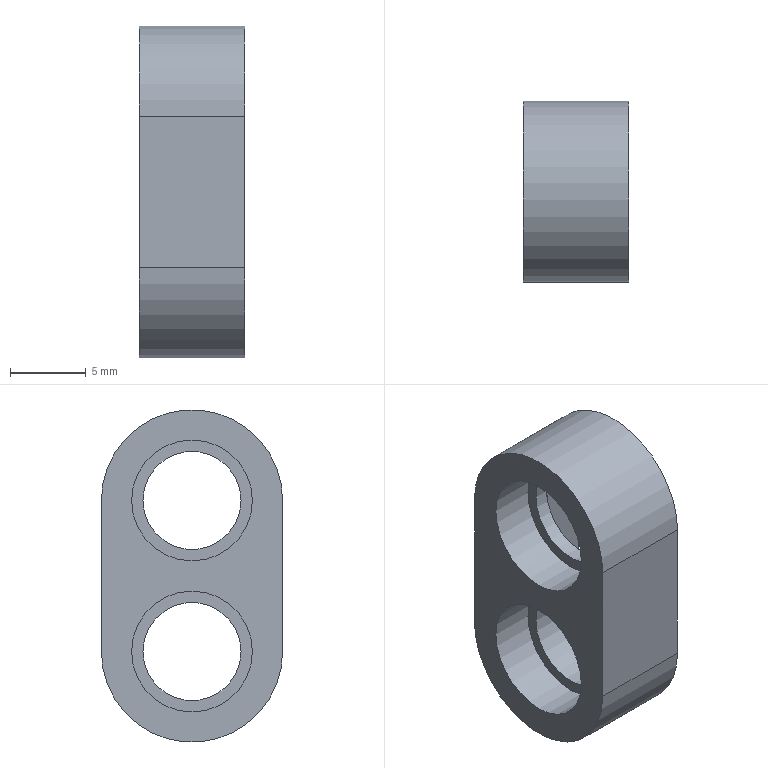Part | STEP file | 1-26.3 | 1 solid | 15 faces | box 7 x 12 x 22 mm | volume 969.173 mm3 | plane 9 | cylinder 6 | commonest cylinder face diameters 6.5 x2 8 x2 12 x2
STEP:
#1=CARTESIAN_POINT('',(0.,0.,0.));
#2=DIRECTION('',(0.,0.,1.));
#3=DIRECTION('',(1.,0.,0.));
#4=AXIS2_PLACEMENT_3D('',#1,#2,#3);
#5=CARTESIAN_POINT('',(0.,6.,5.));
#6=VERTEX_POINT('',#5);
#7=CARTESIAN_POINT('',(-7.,6.,5.));
#8=VERTEX_POINT('',#7);
#9=CARTESIAN_POINT('',(0.,6.,5.));
#10=DIRECTION('',(-1.,0.,0.));
#11=VECTOR('',#10,1.);
#12=LINE('',#9,#11);
#13=CARTESIAN_POINT('',(0.,0.,5.));
#14=DIRECTION('',(-1.,0.,0.));
#15=DIRECTION('',(0.,1.,0.));
#16=AXIS2_PLACEMENT_3D('',#13,#14,#15);
#17=CYLINDRICAL_SURFACE('',#16,6.);
#18=CARTESIAN_POINT('',(6.283,0.));
#19=DIRECTION('',(0.,1.));
#20=VECTOR('',#19,1.);
#21=LINE('',#18,#20);
#22=(GEOMETRIC_REPRESENTATION_CONTEXT(2)PARAMETRIC_REPRESENTATION_CONTEXT()REPRESENTATION_CONTEXT('',''));
#23=DEFINITIONAL_REPRESENTATION('',(#21),#22);
#24=PCURVE('',#17,#23);
#25=CARTESIAN_POINT('',(-3.5,6.,0.));
#26=DIRECTION('',(0.,-1.,0.));
#27=DIRECTION('',(0.,0.,1.));
#28=AXIS2_PLACEMENT_3D('',#25,#26,#27);
#29=PLANE('',#28);
#30=CARTESIAN_POINT('',(5.,-3.5));
#31=DIRECTION('',(0.,1.));
#32=VECTOR('',#31,1.);
#33=LINE('',#30,#32);
#34=(GEOMETRIC_REPRESENTATION_CONTEXT(2)PARAMETRIC_REPRESENTATION_CONTEXT()REPRESENTATION_CONTEXT('',''));
#35=DEFINITIONAL_REPRESENTATION('',(#33),#34);
#36=PCURVE('',#29,#35);
#37=SURFACE_CURVE('',#12,(#24,#36),.PCURVE_S1.);
#38=EDGE_CURVE('',#6,#8,#37,.T.);
#39=ORIENTED_EDGE('',*,*,#38,.T.);
#40=CARTESIAN_POINT('',(-7.,-6.,5.));
#41=VERTEX_POINT('',#40);
#42=CARTESIAN_POINT('',(-7.,0.,5.));
#43=DIRECTION('',(1.,0.,0.));
#44=DIRECTION('',(0.,1.,0.));
#45=AXIS2_PLACEMENT_3D('',#42,#43,#44);
#46=CIRCLE('',#45,6.);
#47=CARTESIAN_POINT('',(6.283,7.));
#48=DIRECTION('',(-1.,0.));
#49=VECTOR('',#48,1.);
#50=LINE('',#47,#49);
#51=(GEOMETRIC_REPRESENTATION_CONTEXT(2)PARAMETRIC_REPRESENTATION_CONTEXT()REPRESENTATION_CONTEXT('',''));
#52=DEFINITIONAL_REPRESENTATION('',(#50),#51);
#53=PCURVE('',#17,#52);
#54=CARTESIAN_POINT('',(-7.,5.,0.));
#55=DIRECTION('',(1.,0.,0.));
#56=DIRECTION('',(0.,0.,-1.));
#57=AXIS2_PLACEMENT_3D('',#54,#55,#56);
#58=PLANE('',#57);
#59=CARTESIAN_POINT('',(-5.,-5.));
#60=DIRECTION('',(0.,1.));
#61=AXIS2_PLACEMENT_2D('',#59,#60);
#62=CIRCLE('',#61,6.);
#63=(GEOMETRIC_REPRESENTATION_CONTEXT(2)PARAMETRIC_REPRESENTATION_CONTEXT()REPRESENTATION_CONTEXT('',''));
#64=DEFINITIONAL_REPRESENTATION('',(#62),#63);
#65=PCURVE('',#58,#64);
#66=SURFACE_CURVE('',#46,(#53,#65),.PCURVE_S1.);
#67=EDGE_CURVE('',#8,#41,#66,.T.);
#68=ORIENTED_EDGE('',*,*,#67,.T.);
#69=CARTESIAN_POINT('',(0.,-6.,5.));
#70=VERTEX_POINT('',#69);
#71=CARTESIAN_POINT('',(0.,-6.,5.));
#72=DIRECTION('',(-1.,0.,0.));
#73=VECTOR('',#72,1.);
#74=LINE('',#71,#73);
#75=CARTESIAN_POINT('',(3.142,0.));
#76=DIRECTION('',(0.,1.));
#77=VECTOR('',#76,1.);
#78=LINE('',#75,#77);
#79=(GEOMETRIC_REPRESENTATION_CONTEXT(2)PARAMETRIC_REPRESENTATION_CONTEXT()REPRESENTATION_CONTEXT('',''));
#80=DEFINITIONAL_REPRESENTATION('',(#78),#79);
#81=PCURVE('',#17,#80);
#82=CARTESIAN_POINT('',(-3.5,-6.,0.));
#83=DIRECTION('',(0.,1.,0.));
#84=DIRECTION('',(0.,0.,-1.));
#85=AXIS2_PLACEMENT_3D('',#82,#83,#84);
#86=PLANE('',#85);
#87=CARTESIAN_POINT('',(-5.,-3.5));
#88=DIRECTION('',(0.,1.));
#89=VECTOR('',#88,1.);
#90=LINE('',#87,#89);
#91=(GEOMETRIC_REPRESENTATION_CONTEXT(2)PARAMETRIC_REPRESENTATION_CONTEXT()REPRESENTATION_CONTEXT('',''));
#92=DEFINITIONAL_REPRESENTATION('',(#90),#91);
#93=PCURVE('',#86,#92);
#94=SURFACE_CURVE('',#74,(#81,#93),.PCURVE_S1.);
#95=EDGE_CURVE('',#70,#41,#94,.T.);
#96=ORIENTED_EDGE('',*,*,#95,.F.);
#97=CARTESIAN_POINT('',(0.,0.,5.));
#98=DIRECTION('',(1.,0.,0.));
#99=DIRECTION('',(0.,1.,0.));
#100=AXIS2_PLACEMENT_3D('',#97,#98,#99);
#101=CIRCLE('',#100,6.);
#102=CARTESIAN_POINT('',(6.283,0.));
#103=DIRECTION('',(-1.,0.));
#104=VECTOR('',#103,1.);
#105=LINE('',#102,#104);
#106=(GEOMETRIC_REPRESENTATION_CONTEXT(2)PARAMETRIC_REPRESENTATION_CONTEXT()REPRESENTATION_CONTEXT('',''));
#107=DEFINITIONAL_REPRESENTATION('',(#105),#106);
#108=PCURVE('',#17,#107);
#109=CARTESIAN_POINT('',(0.,5.,0.));
#110=DIRECTION('',(1.,0.,0.));
#111=DIRECTION('',(0.,0.,-1.));
#112=AXIS2_PLACEMENT_3D('',#109,#110,#111);
#113=PLANE('',#112);
#114=CARTESIAN_POINT('',(-5.,-5.));
#115=DIRECTION('',(0.,1.));
#116=AXIS2_PLACEMENT_2D('',#114,#115);
#117=CIRCLE('',#116,6.);
#118=(GEOMETRIC_REPRESENTATION_CONTEXT(2)PARAMETRIC_REPRESENTATION_CONTEXT()REPRESENTATION_CONTEXT('',''));
#119=DEFINITIONAL_REPRESENTATION('',(#117),#118);
#120=PCURVE('',#113,#119);
#121=SURFACE_CURVE('',#101,(#108,#120),.PCURVE_S1.);
#122=EDGE_CURVE('',#6,#70,#121,.T.);
#123=ORIENTED_EDGE('',*,*,#122,.F.);
#124=EDGE_LOOP('',(#39,#68,#96,#123));
#125=FACE_BOUND('',#124,.T.);
#126=ADVANCED_FACE('',(#125),#17,.T.);
#127=CARTESIAN_POINT('',(0.,-6.,-5.));
#128=VERTEX_POINT('',#127);
#129=CARTESIAN_POINT('',(0.,-6.,5.));
#130=DIRECTION('',(0.,0.,-1.));
#131=VECTOR('',#130,1.);
#132=LINE('',#129,#131);
#133=CARTESIAN_POINT('',(-5.,-3.5));
#134=DIRECTION('',(1.,0.));
#135=VECTOR('',#134,1.);
#136=LINE('',#133,#135);
#137=(GEOMETRIC_REPRESENTATION_CONTEXT(2)PARAMETRIC_REPRESENTATION_CONTEXT()REPRESENTATION_CONTEXT('',''));
#138=DEFINITIONAL_REPRESENTATION('',(#136),#137);
#139=PCURVE('',#86,#138);
#140=CARTESIAN_POINT('',(-5.,-11.));
#141=DIRECTION('',(1.,0.));
#142=VECTOR('',#141,1.);
#143=LINE('',#140,#142);
#144=(GEOMETRIC_REPRESENTATION_CONTEXT(2)PARAMETRIC_REPRESENTATION_CONTEXT()REPRESENTATION_CONTEXT('',''));
#145=DEFINITIONAL_REPRESENTATION('',(#143),#144);
#146=PCURVE('',#113,#145);
#147=SURFACE_CURVE('',#132,(#139,#146),.PCURVE_S1.);
#148=EDGE_CURVE('',#70,#128,#147,.T.);
#149=ORIENTED_EDGE('',*,*,#148,.T.);
#150=CARTESIAN_POINT('',(-7.,-6.,-5.));
#151=VERTEX_POINT('',#150);
#152=CARTESIAN_POINT('',(0.,-6.,-5.));
#153=DIRECTION('',(-1.,0.,0.));
#154=VECTOR('',#153,1.);
#155=LINE('',#152,#154);
#156=CARTESIAN_POINT('',(5.,-3.5));
#157=DIRECTION('',(0.,1.));
#158=VECTOR('',#157,1.);
#159=LINE('',#156,#158);
#160=(GEOMETRIC_REPRESENTATION_CONTEXT(2)PARAMETRIC_REPRESENTATION_CONTEXT()REPRESENTATION_CONTEXT('',''));
#161=DEFINITIONAL_REPRESENTATION('',(#159),#160);
#162=PCURVE('',#86,#161);
#163=CARTESIAN_POINT('',(0.,0.,-5.));
#164=DIRECTION('',(-1.,0.,0.));
#165=DIRECTION('',(0.,-1.,0.));
#166=AXIS2_PLACEMENT_3D('',#163,#164,#165);
#167=CYLINDRICAL_SURFACE('',#166,6.);
#168=CARTESIAN_POINT('',(6.283,0.));
#169=DIRECTION('',(0.,1.));
#170=VECTOR('',#169,1.);
#171=LINE('',#168,#170);
#172=(GEOMETRIC_REPRESENTATION_CONTEXT(2)PARAMETRIC_REPRESENTATION_CONTEXT()REPRESENTATION_CONTEXT('',''));
#173=DEFINITIONAL_REPRESENTATION('',(#171),#172);
#174=PCURVE('',#167,#173);
#175=SURFACE_CURVE('',#155,(#162,#174),.PCURVE_S1.);
#176=EDGE_CURVE('',#128,#151,#175,.T.);
#177=ORIENTED_EDGE('',*,*,#176,.T.);
#178=CARTESIAN_POINT('',(-7.,-6.,5.));
#179=DIRECTION('',(0.,0.,-1.));
#180=VECTOR('',#179,1.);
#181=LINE('',#178,#180);
#182=CARTESIAN_POINT('',(-5.,3.5));
#183=DIRECTION('',(1.,0.));
#184=VECTOR('',#183,1.);
#185=LINE('',#182,#184);
#186=(GEOMETRIC_REPRESENTATION_CONTEXT(2)PARAMETRIC_REPRESENTATION_CONTEXT()REPRESENTATION_CONTEXT('',''));
#187=DEFINITIONAL_REPRESENTATION('',(#185),#186);
#188=PCURVE('',#86,#187);
#189=CARTESIAN_POINT('',(-5.,-11.));
#190=DIRECTION('',(1.,0.));
#191=VECTOR('',#190,1.);
#192=LINE('',#189,#191);
#193=(GEOMETRIC_REPRESENTATION_CONTEXT(2)PARAMETRIC_REPRESENTATION_CONTEXT()REPRESENTATION_CONTEXT('',''));
#194=DEFINITIONAL_REPRESENTATION('',(#192),#193);
#195=PCURVE('',#58,#194);
#196=SURFACE_CURVE('',#181,(#188,#195),.PCURVE_S1.);
#197=EDGE_CURVE('',#41,#151,#196,.T.);
#198=ORIENTED_EDGE('',*,*,#197,.F.);
#199=ORIENTED_EDGE('',*,*,#95,.F.);
#200=EDGE_LOOP('',(#149,#177,#198,#199));
#201=FACE_BOUND('',#200,.F.);
#202=ADVANCED_FACE('',(#201),#86,.F.);
#203=ORIENTED_EDGE('',*,*,#176,.T.);
#204=CARTESIAN_POINT('',(-7.,6.,-5.));
#205=VERTEX_POINT('',#204);
#206=CARTESIAN_POINT('',(-7.,0.,-5.));
#207=DIRECTION('',(1.,0.,0.));
#208=DIRECTION('',(0.,-1.,0.));
#209=AXIS2_PLACEMENT_3D('',#206,#207,#208);
#210=CIRCLE('',#209,6.);
#211=CARTESIAN_POINT('',(6.283,7.));
#212=DIRECTION('',(-1.,0.));
#213=VECTOR('',#212,1.);
#214=LINE('',#211,#213);
#215=(GEOMETRIC_REPRESENTATION_CONTEXT(2)PARAMETRIC_REPRESENTATION_CONTEXT()REPRESENTATION_CONTEXT('',''));
#216=DEFINITIONAL_REPRESENTATION('',(#214),#215);
#217=PCURVE('',#167,#216);
#218=CARTESIAN_POINT('',(5.,-5.));
#219=DIRECTION('',(0.,-1.));
#220=AXIS2_PLACEMENT_2D('',#218,#219);
#221=CIRCLE('',#220,6.);
#222=(GEOMETRIC_REPRESENTATION_CONTEXT(2)PARAMETRIC_REPRESENTATION_CONTEXT()REPRESENTATION_CONTEXT('',''));
#223=DEFINITIONAL_REPRESENTATION('',(#221),#222);
#224=PCURVE('',#58,#223);
#225=SURFACE_CURVE('',#210,(#217,#224),.PCURVE_S1.);
#226=EDGE_CURVE('',#151,#205,#225,.T.);
#227=ORIENTED_EDGE('',*,*,#226,.T.);
#228=CARTESIAN_POINT('',(0.,6.,-5.));
#229=VERTEX_POINT('',#228);
#230=CARTESIAN_POINT('',(0.,6.,-5.));
#231=DIRECTION('',(-1.,0.,0.));
#232=VECTOR('',#231,1.);
#233=LINE('',#230,#232);
#234=CARTESIAN_POINT('',(3.142,0.));
#235=DIRECTION('',(0.,1.));
#236=VECTOR('',#235,1.);
#237=LINE('',#234,#236);
#238=(GEOMETRIC_REPRESENTATION_CONTEXT(2)PARAMETRIC_REPRESENTATION_CONTEXT()REPRESENTATION_CONTEXT('',''));
#239=DEFINITIONAL_REPRESENTATION('',(#237),#238);
#240=PCURVE('',#167,#239);
#241=CARTESIAN_POINT('',(-5.,-3.5));
#242=DIRECTION('',(0.,1.));
#243=VECTOR('',#242,1.);
#244=LINE('',#241,#243);
#245=(GEOMETRIC_REPRESENTATION_CONTEXT(2)PARAMETRIC_REPRESENTATION_CONTEXT()REPRESENTATION_CONTEXT('',''));
#246=DEFINITIONAL_REPRESENTATION('',(#244),#245);
#247=PCURVE('',#29,#246);
#248=SURFACE_CURVE('',#233,(#240,#247),.PCURVE_S1.);
#249=EDGE_CURVE('',#229,#205,#248,.T.);
#250=ORIENTED_EDGE('',*,*,#249,.F.);
#251=CARTESIAN_POINT('',(0.,0.,-5.));
#252=DIRECTION('',(1.,0.,0.));
#253=DIRECTION('',(0.,-1.,0.));
#254=AXIS2_PLACEMENT_3D('',#251,#252,#253);
#255=CIRCLE('',#254,6.);
#256=CARTESIAN_POINT('',(6.283,0.));
#257=DIRECTION('',(-1.,0.));
#258=VECTOR('',#257,1.);
#259=LINE('',#256,#258);
#260=(GEOMETRIC_REPRESENTATION_CONTEXT(2)PARAMETRIC_REPRESENTATION_CONTEXT()REPRESENTATION_CONTEXT('',''));
#261=DEFINITIONAL_REPRESENTATION('',(#259),#260);
#262=PCURVE('',#167,#261);
#263=CARTESIAN_POINT('',(5.,-5.));
#264=DIRECTION('',(0.,-1.));
#265=AXIS2_PLACEMENT_2D('',#263,#264);
#266=CIRCLE('',#265,6.);
#267=(GEOMETRIC_REPRESENTATION_CONTEXT(2)PARAMETRIC_REPRESENTATION_CONTEXT()REPRESENTATION_CONTEXT('',''));
#268=DEFINITIONAL_REPRESENTATION('',(#266),#267);
#269=PCURVE('',#113,#268);
#270=SURFACE_CURVE('',#255,(#262,#269),.PCURVE_S1.);
#271=EDGE_CURVE('',#128,#229,#270,.T.);
#272=ORIENTED_EDGE('',*,*,#271,.F.);
#273=EDGE_LOOP('',(#203,#227,#250,#272));
#274=FACE_BOUND('',#273,.T.);
#275=ADVANCED_FACE('',(#274),#167,.T.);
#276=CARTESIAN_POINT('',(0.,6.,-5.));
#277=DIRECTION('',(0.,0.,1.));
#278=VECTOR('',#277,1.);
#279=LINE('',#276,#278);
#280=CARTESIAN_POINT('',(-5.,-3.5));
#281=DIRECTION('',(1.,0.));
#282=VECTOR('',#281,1.);
#283=LINE('',#280,#282);
#284=(GEOMETRIC_REPRESENTATION_CONTEXT(2)PARAMETRIC_REPRESENTATION_CONTEXT()REPRESENTATION_CONTEXT('',''));
#285=DEFINITIONAL_REPRESENTATION('',(#283),#284);
#286=PCURVE('',#29,#285);
#287=CARTESIAN_POINT('',(5.,1.));
#288=DIRECTION('',(-1.,0.));
#289=VECTOR('',#288,1.);
#290=LINE('',#287,#289);
#291=(GEOMETRIC_REPRESENTATION_CONTEXT(2)PARAMETRIC_REPRESENTATION_CONTEXT()REPRESENTATION_CONTEXT('',''));
#292=DEFINITIONAL_REPRESENTATION('',(#290),#291);
#293=PCURVE('',#113,#292);
#294=SURFACE_CURVE('',#279,(#286,#293),.PCURVE_S1.);
#295=EDGE_CURVE('',#229,#6,#294,.T.);
#296=ORIENTED_EDGE('',*,*,#295,.T.);
#297=ORIENTED_EDGE('',*,*,#38,.T.);
#298=CARTESIAN_POINT('',(-7.,6.,-5.));
#299=DIRECTION('',(0.,0.,1.));
#300=VECTOR('',#299,1.);
#301=LINE('',#298,#300);
#302=CARTESIAN_POINT('',(-5.,3.5));
#303=DIRECTION('',(1.,0.));
#304=VECTOR('',#303,1.);
#305=LINE('',#302,#304);
#306=(GEOMETRIC_REPRESENTATION_CONTEXT(2)PARAMETRIC_REPRESENTATION_CONTEXT()REPRESENTATION_CONTEXT('',''));
#307=DEFINITIONAL_REPRESENTATION('',(#305),#306);
#308=PCURVE('',#29,#307);
#309=CARTESIAN_POINT('',(5.,1.));
#310=DIRECTION('',(-1.,0.));
#311=VECTOR('',#310,1.);
#312=LINE('',#309,#311);
#313=(GEOMETRIC_REPRESENTATION_CONTEXT(2)PARAMETRIC_REPRESENTATION_CONTEXT()REPRESENTATION_CONTEXT('',''));
#314=DEFINITIONAL_REPRESENTATION('',(#312),#313);
#315=PCURVE('',#58,#314);
#316=SURFACE_CURVE('',#301,(#308,#315),.PCURVE_S1.);
#317=EDGE_CURVE('',#205,#8,#316,.T.);
#318=ORIENTED_EDGE('',*,*,#317,.F.);
#319=ORIENTED_EDGE('',*,*,#249,.F.);
#320=EDGE_LOOP('',(#296,#297,#318,#319));
#321=FACE_BOUND('',#320,.F.);
#322=ADVANCED_FACE('',(#321),#29,.F.);
#323=ORIENTED_EDGE('',*,*,#122,.T.);
#324=ORIENTED_EDGE('',*,*,#148,.T.);
#325=ORIENTED_EDGE('',*,*,#271,.T.);
#326=ORIENTED_EDGE('',*,*,#295,.T.);
#327=EDGE_LOOP('',(#323,#324,#325,#326));
#328=FACE_BOUND('',#327,.T.);
#329=CARTESIAN_POINT('',(0.,3.25,-5.));
#330=VERTEX_POINT('',#329);
#331=CARTESIAN_POINT('',(0.,-3.25,-5.));
#332=VERTEX_POINT('',#331);
#333=CARTESIAN_POINT('',(0.,0.,-5.));
#334=DIRECTION('',(-1.,0.,0.));
#335=DIRECTION('',(0.,1.,0.));
#336=AXIS2_PLACEMENT_3D('',#333,#334,#335);
#337=CIRCLE('',#336,3.25);
#338=CARTESIAN_POINT('',(5.,-1.75));
#339=CARTESIAN_POINT('',(10.629,-1.75));
#340=CARTESIAN_POINT('',(7.815,-6.625));
#341=CARTESIAN_POINT('',(5.,-11.5));
#342=CARTESIAN_POINT('',(2.185,-6.625));
#343=CARTESIAN_POINT('',(-0.6292,-1.75));
#344=CARTESIAN_POINT('',(5.,-1.75));
#345=(BOUNDED_CURVE()B_SPLINE_CURVE(2,(#338,#339,#340,#341,#342,#343,#344),.UNSPECIFIED.,.T.,.F.)B_SPLINE_CURVE_WITH_KNOTS((1,2,2,2,2,1),(-2.094,0.,2.094,4.189,6.283,8.378),.UNSPECIFIED.)CURVE()GEOMETRIC_REPRESENTATION_ITEM()RATIONAL_B_SPLINE_CURVE((1.,0.5,1.,0.5,1.,0.5,1.))REPRESENTATION_ITEM(''));
#346=(GEOMETRIC_REPRESENTATION_CONTEXT(2)PARAMETRIC_REPRESENTATION_CONTEXT()REPRESENTATION_CONTEXT('',''));
#347=DEFINITIONAL_REPRESENTATION('',(#345),#346);
#348=PCURVE('',#113,#347);
#349=CARTESIAN_POINT('',(0.,0.,-5.));
#350=DIRECTION('',(-1.,0.,0.));
#351=DIRECTION('',(0.,-1.,0.));
#352=AXIS2_PLACEMENT_3D('',#349,#350,#351);
#353=CYLINDRICAL_SURFACE('',#352,3.25);
#354=CARTESIAN_POINT('',(3.142,0.));
#355=DIRECTION('',(1.,0.));
#356=VECTOR('',#355,1.);
#357=LINE('',#354,#356);
#358=(GEOMETRIC_REPRESENTATION_CONTEXT(2)PARAMETRIC_REPRESENTATION_CONTEXT()REPRESENTATION_CONTEXT('',''));
#359=DEFINITIONAL_REPRESENTATION('',(#357),#358);
#360=PCURVE('',#353,#359);
#361=SURFACE_CURVE('',#337,(#348,#360),.PCURVE_S1.);
#362=EDGE_CURVE('',#330,#332,#361,.T.);
#363=ORIENTED_EDGE('',*,*,#362,.T.);
#364=CARTESIAN_POINT('',(0.,-3.25,5.));
#365=VERTEX_POINT('',#364);
#366=CARTESIAN_POINT('',(0.,-3.25,5.));
#367=DIRECTION('',(0.,0.,-1.));
#368=VECTOR('',#367,1.);
#369=LINE('',#366,#368);
#370=CARTESIAN_POINT('',(-5.,-8.25));
#371=DIRECTION('',(1.,0.));
#372=VECTOR('',#371,1.);
#373=LINE('',#370,#372);
#374=(GEOMETRIC_REPRESENTATION_CONTEXT(2)PARAMETRIC_REPRESENTATION_CONTEXT()REPRESENTATION_CONTEXT('',''));
#375=DEFINITIONAL_REPRESENTATION('',(#373),#374);
#376=PCURVE('',#113,#375);
#377=CARTESIAN_POINT('',(-1.5,-3.25,0.));
#378=DIRECTION('',(0.,1.,0.));
#379=DIRECTION('',(0.,0.,-1.));
#380=AXIS2_PLACEMENT_3D('',#377,#378,#379);
#381=PLANE('',#380);
#382=CARTESIAN_POINT('',(-5.,-1.5));
#383=DIRECTION('',(1.,0.));
#384=VECTOR('',#383,1.);
#385=LINE('',#382,#384);
#386=(GEOMETRIC_REPRESENTATION_CONTEXT(2)PARAMETRIC_REPRESENTATION_CONTEXT()REPRESENTATION_CONTEXT('',''));
#387=DEFINITIONAL_REPRESENTATION('',(#385),#386);
#388=PCURVE('',#381,#387);
#389=SURFACE_CURVE('',#369,(#376,#388),.PCURVE_S1.);
#390=EDGE_CURVE('',#365,#332,#389,.T.);
#391=ORIENTED_EDGE('',*,*,#390,.F.);
#392=CARTESIAN_POINT('',(0.,3.25,5.));
#393=VERTEX_POINT('',#392);
#394=CARTESIAN_POINT('',(0.,0.,5.));
#395=DIRECTION('',(-1.,0.,0.));
#396=DIRECTION('',(0.,-1.,0.));
#397=AXIS2_PLACEMENT_3D('',#394,#395,#396);
#398=CIRCLE('',#397,3.25);
#399=CARTESIAN_POINT('',(-5.,-8.25));
#400=CARTESIAN_POINT('',(-10.629,-8.25));
#401=CARTESIAN_POINT('',(-7.815,-3.375));
#402=CARTESIAN_POINT('',(-5.,1.5));
#403=CARTESIAN_POINT('',(-2.185,-3.375));
#404=CARTESIAN_POINT('',(0.6292,-8.25));
#405=CARTESIAN_POINT('',(-5.,-8.25));
#406=(BOUNDED_CURVE()B_SPLINE_CURVE(2,(#399,#400,#401,#402,#403,#404,#405),.UNSPECIFIED.,.T.,.F.)B_SPLINE_CURVE_WITH_KNOTS((1,2,2,2,2,1),(-2.094,0.,2.094,4.189,6.283,8.378),.UNSPECIFIED.)CURVE()GEOMETRIC_REPRESENTATION_ITEM()RATIONAL_B_SPLINE_CURVE((1.,0.5,1.,0.5,1.,0.5,1.))REPRESENTATION_ITEM(''));
#407=(GEOMETRIC_REPRESENTATION_CONTEXT(2)PARAMETRIC_REPRESENTATION_CONTEXT()REPRESENTATION_CONTEXT('',''));
#408=DEFINITIONAL_REPRESENTATION('',(#406),#407);
#409=PCURVE('',#113,#408);
#410=CARTESIAN_POINT('',(0.,0.,5.));
#411=DIRECTION('',(-1.,0.,0.));
#412=DIRECTION('',(0.,1.,0.));
#413=AXIS2_PLACEMENT_3D('',#410,#411,#412);
#414=CYLINDRICAL_SURFACE('',#413,3.25);
#415=CARTESIAN_POINT('',(3.142,0.));
#416=DIRECTION('',(1.,0.));
#417=VECTOR('',#416,1.);
#418=LINE('',#415,#417);
#419=(GEOMETRIC_REPRESENTATION_CONTEXT(2)PARAMETRIC_REPRESENTATION_CONTEXT()REPRESENTATION_CONTEXT('',''));
#420=DEFINITIONAL_REPRESENTATION('',(#418),#419);
#421=PCURVE('',#414,#420);
#422=SURFACE_CURVE('',#398,(#409,#421),.PCURVE_S1.);
#423=EDGE_CURVE('',#365,#393,#422,.T.);
#424=ORIENTED_EDGE('',*,*,#423,.T.);
#425=CARTESIAN_POINT('',(0.,3.25,-5.));
#426=DIRECTION('',(0.,0.,1.));
#427=VECTOR('',#426,1.);
#428=LINE('',#425,#427);
#429=CARTESIAN_POINT('',(5.,-1.75));
#430=DIRECTION('',(-1.,0.));
#431=VECTOR('',#430,1.);
#432=LINE('',#429,#431);
#433=(GEOMETRIC_REPRESENTATION_CONTEXT(2)PARAMETRIC_REPRESENTATION_CONTEXT()REPRESENTATION_CONTEXT('',''));
#434=DEFINITIONAL_REPRESENTATION('',(#432),#433);
#435=PCURVE('',#113,#434);
#436=CARTESIAN_POINT('',(-1.5,3.25,0.));
#437=DIRECTION('',(0.,-1.,0.));
#438=DIRECTION('',(0.,0.,1.));
#439=AXIS2_PLACEMENT_3D('',#436,#437,#438);
#440=PLANE('',#439);
#441=CARTESIAN_POINT('',(-5.,-1.5));
#442=DIRECTION('',(1.,0.));
#443=VECTOR('',#442,1.);
#444=LINE('',#441,#443);
#445=(GEOMETRIC_REPRESENTATION_CONTEXT(2)PARAMETRIC_REPRESENTATION_CONTEXT()REPRESENTATION_CONTEXT('',''));
#446=DEFINITIONAL_REPRESENTATION('',(#444),#445);
#447=PCURVE('',#440,#446);
#448=SURFACE_CURVE('',#428,(#435,#447),.PCURVE_S1.);
#449=EDGE_CURVE('',#330,#393,#448,.T.);
#450=ORIENTED_EDGE('',*,*,#449,.F.);
#451=EDGE_LOOP('',(#363,#391,#424,#450));
#452=FACE_BOUND('',#451,.T.);
#453=ADVANCED_FACE('',(#328,#452),#113,.T.);
#454=ORIENTED_EDGE('',*,*,#390,.T.);
#455=CARTESIAN_POINT('',(-3.,-3.25,-5.));
#456=VERTEX_POINT('',#455);
#457=CARTESIAN_POINT('',(0.,-3.25,-5.));
#458=DIRECTION('',(-1.,0.,0.));
#459=VECTOR('',#458,1.);
#460=LINE('',#457,#459);
#461=CARTESIAN_POINT('',(5.,-1.5));
#462=DIRECTION('',(0.,1.));
#463=VECTOR('',#462,1.);
#464=LINE('',#461,#463);
#465=(GEOMETRIC_REPRESENTATION_CONTEXT(2)PARAMETRIC_REPRESENTATION_CONTEXT()REPRESENTATION_CONTEXT('',''));
#466=DEFINITIONAL_REPRESENTATION('',(#464),#465);
#467=PCURVE('',#381,#466);
#468=CARTESIAN_POINT('',(6.283,0.));
#469=DIRECTION('',(0.,1.));
#470=VECTOR('',#469,1.);
#471=LINE('',#468,#470);
#472=(GEOMETRIC_REPRESENTATION_CONTEXT(2)PARAMETRIC_REPRESENTATION_CONTEXT()REPRESENTATION_CONTEXT('',''));
#473=DEFINITIONAL_REPRESENTATION('',(#471),#472);
#474=PCURVE('',#353,#473);
#475=SURFACE_CURVE('',#460,(#467,#474),.PCURVE_S1.);
#476=EDGE_CURVE('',#332,#456,#475,.T.);
#477=ORIENTED_EDGE('',*,*,#476,.T.);
#478=CARTESIAN_POINT('',(-3.,-3.25,5.));
#479=VERTEX_POINT('',#478);
#480=CARTESIAN_POINT('',(-3.,-3.25,5.));
#481=DIRECTION('',(0.,0.,-1.));
#482=VECTOR('',#481,1.);
#483=LINE('',#480,#482);
#484=CARTESIAN_POINT('',(-5.,1.5));
#485=DIRECTION('',(1.,0.));
#486=VECTOR('',#485,1.);
#487=LINE('',#484,#486);
#488=(GEOMETRIC_REPRESENTATION_CONTEXT(2)PARAMETRIC_REPRESENTATION_CONTEXT()REPRESENTATION_CONTEXT('',''));
#489=DEFINITIONAL_REPRESENTATION('',(#487),#488);
#490=PCURVE('',#381,#489);
#491=CARTESIAN_POINT('',(-3.,5.,0.));
#492=DIRECTION('',(1.,0.,0.));
#493=DIRECTION('',(0.,0.,-1.));
#494=AXIS2_PLACEMENT_3D('',#491,#492,#493);
#495=PLANE('',#494);
#496=CARTESIAN_POINT('',(-5.,-8.25));
#497=DIRECTION('',(1.,0.));
#498=VECTOR('',#497,1.);
#499=LINE('',#496,#498);
#500=(GEOMETRIC_REPRESENTATION_CONTEXT(2)PARAMETRIC_REPRESENTATION_CONTEXT()REPRESENTATION_CONTEXT('',''));
#501=DEFINITIONAL_REPRESENTATION('',(#499),#500);
#502=PCURVE('',#495,#501);
#503=SURFACE_CURVE('',#483,(#490,#502),.PCURVE_S1.);
#504=EDGE_CURVE('',#479,#456,#503,.T.);
#505=ORIENTED_EDGE('',*,*,#504,.F.);
#506=CARTESIAN_POINT('',(0.,-3.25,5.));
#507=DIRECTION('',(-1.,0.,0.));
#508=VECTOR('',#507,1.);
#509=LINE('',#506,#508);
#510=CARTESIAN_POINT('',(-5.,-1.5));
#511=DIRECTION('',(0.,1.));
#512=VECTOR('',#511,1.);
#513=LINE('',#510,#512);
#514=(GEOMETRIC_REPRESENTATION_CONTEXT(2)PARAMETRIC_REPRESENTATION_CONTEXT()REPRESENTATION_CONTEXT('',''));
#515=DEFINITIONAL_REPRESENTATION('',(#513),#514);
#516=PCURVE('',#381,#515);
#517=CARTESIAN_POINT('',(3.142,0.));
#518=DIRECTION('',(0.,1.));
#519=VECTOR('',#518,1.);
#520=LINE('',#517,#519);
#521=(GEOMETRIC_REPRESENTATION_CONTEXT(2)PARAMETRIC_REPRESENTATION_CONTEXT()REPRESENTATION_CONTEXT('',''));
#522=DEFINITIONAL_REPRESENTATION('',(#520),#521);
#523=PCURVE('',#414,#522);
#524=SURFACE_CURVE('',#509,(#516,#523),.PCURVE_S1.);
#525=EDGE_CURVE('',#365,#479,#524,.T.);
#526=ORIENTED_EDGE('',*,*,#525,.F.);
#527=EDGE_LOOP('',(#454,#477,#505,#526));
#528=FACE_BOUND('',#527,.T.);
#529=ADVANCED_FACE('',(#528),#381,.T.);
#530=ORIENTED_EDGE('',*,*,#449,.T.);
#531=CARTESIAN_POINT('',(-3.,3.25,5.));
#532=VERTEX_POINT('',#531);
#533=CARTESIAN_POINT('',(0.,3.25,5.));
#534=DIRECTION('',(-1.,0.,0.));
#535=VECTOR('',#534,1.);
#536=LINE('',#533,#535);
#537=CARTESIAN_POINT('',(5.,-1.5));
#538=DIRECTION('',(0.,1.));
#539=VECTOR('',#538,1.);
#540=LINE('',#537,#539);
#541=(GEOMETRIC_REPRESENTATION_CONTEXT(2)PARAMETRIC_REPRESENTATION_CONTEXT()REPRESENTATION_CONTEXT('',''));
#542=DEFINITIONAL_REPRESENTATION('',(#540),#541);
#543=PCURVE('',#440,#542);
#544=CARTESIAN_POINT('',(6.283,0.));
#545=DIRECTION('',(0.,1.));
#546=VECTOR('',#545,1.);
#547=LINE('',#544,#546);
#548=(GEOMETRIC_REPRESENTATION_CONTEXT(2)PARAMETRIC_REPRESENTATION_CONTEXT()REPRESENTATION_CONTEXT('',''));
#549=DEFINITIONAL_REPRESENTATION('',(#547),#548);
#550=PCURVE('',#414,#549);
#551=SURFACE_CURVE('',#536,(#543,#550),.PCURVE_S1.);
#552=EDGE_CURVE('',#393,#532,#551,.T.);
#553=ORIENTED_EDGE('',*,*,#552,.T.);
#554=CARTESIAN_POINT('',(-3.,3.25,-5.));
#555=VERTEX_POINT('',#554);
#556=CARTESIAN_POINT('',(-3.,3.25,-5.));
#557=DIRECTION('',(0.,0.,1.));
#558=VECTOR('',#557,1.);
#559=LINE('',#556,#558);
#560=CARTESIAN_POINT('',(-5.,1.5));
#561=DIRECTION('',(1.,0.));
#562=VECTOR('',#561,1.);
#563=LINE('',#560,#562);
#564=(GEOMETRIC_REPRESENTATION_CONTEXT(2)PARAMETRIC_REPRESENTATION_CONTEXT()REPRESENTATION_CONTEXT('',''));
#565=DEFINITIONAL_REPRESENTATION('',(#563),#564);
#566=PCURVE('',#440,#565);
#567=CARTESIAN_POINT('',(5.,-1.75));
#568=DIRECTION('',(-1.,0.));
#569=VECTOR('',#568,1.);
#570=LINE('',#567,#569);
#571=(GEOMETRIC_REPRESENTATION_CONTEXT(2)PARAMETRIC_REPRESENTATION_CONTEXT()REPRESENTATION_CONTEXT('',''));
#572=DEFINITIONAL_REPRESENTATION('',(#570),#571);
#573=PCURVE('',#495,#572);
#574=SURFACE_CURVE('',#559,(#566,#573),.PCURVE_S1.);
#575=EDGE_CURVE('',#555,#532,#574,.T.);
#576=ORIENTED_EDGE('',*,*,#575,.F.);
#577=CARTESIAN_POINT('',(0.,3.25,-5.));
#578=DIRECTION('',(-1.,0.,0.));
#579=VECTOR('',#578,1.);
#580=LINE('',#577,#579);
#581=CARTESIAN_POINT('',(-5.,-1.5));
#582=DIRECTION('',(0.,1.));
#583=VECTOR('',#582,1.);
#584=LINE('',#581,#583);
#585=(GEOMETRIC_REPRESENTATION_CONTEXT(2)PARAMETRIC_REPRESENTATION_CONTEXT()REPRESENTATION_CONTEXT('',''));
#586=DEFINITIONAL_REPRESENTATION('',(#584),#585);
#587=PCURVE('',#440,#586);
#588=CARTESIAN_POINT('',(3.142,0.));
#589=DIRECTION('',(0.,1.));
#590=VECTOR('',#589,1.);
#591=LINE('',#588,#590);
#592=(GEOMETRIC_REPRESENTATION_CONTEXT(2)PARAMETRIC_REPRESENTATION_CONTEXT()REPRESENTATION_CONTEXT('',''));
#593=DEFINITIONAL_REPRESENTATION('',(#591),#592);
#594=PCURVE('',#353,#593);
#595=SURFACE_CURVE('',#580,(#587,#594),.PCURVE_S1.);
#596=EDGE_CURVE('',#330,#555,#595,.T.);
#597=ORIENTED_EDGE('',*,*,#596,.F.);
#598=EDGE_LOOP('',(#530,#553,#576,#597));
#599=FACE_BOUND('',#598,.T.);
#600=ADVANCED_FACE('',(#599),#440,.T.);
#601=ORIENTED_EDGE('',*,*,#504,.T.);
#602=CARTESIAN_POINT('',(-3.,0.,-5.));
#603=DIRECTION('',(-1.,0.,0.));
#604=DIRECTION('',(0.,-1.,0.));
#605=AXIS2_PLACEMENT_3D('',#602,#603,#604);
#606=CIRCLE('',#605,3.25);
#607=CARTESIAN_POINT('',(5.,-8.25));
#608=CARTESIAN_POINT('',(-0.6292,-8.25));
#609=CARTESIAN_POINT('',(2.185,-3.375));
#610=CARTESIAN_POINT('',(5.,1.5));
#611=CARTESIAN_POINT('',(7.815,-3.375));
#612=CARTESIAN_POINT('',(10.629,-8.25));
#613=CARTESIAN_POINT('',(5.,-8.25));
#614=(BOUNDED_CURVE()B_SPLINE_CURVE(2,(#607,#608,#609,#610,#611,#612,#613),.UNSPECIFIED.,.T.,.F.)B_SPLINE_CURVE_WITH_KNOTS((1,2,2,2,2,1),(-2.094,0.,2.094,4.189,6.283,8.378),.UNSPECIFIED.)CURVE()GEOMETRIC_REPRESENTATION_ITEM()RATIONAL_B_SPLINE_CURVE((1.,0.5,1.,0.5,1.,0.5,1.))REPRESENTATION_ITEM(''));
#615=(GEOMETRIC_REPRESENTATION_CONTEXT(2)PARAMETRIC_REPRESENTATION_CONTEXT()REPRESENTATION_CONTEXT('',''));
#616=DEFINITIONAL_REPRESENTATION('',(#614),#615);
#617=PCURVE('',#495,#616);
#618=CARTESIAN_POINT('',(0.,3.));
#619=DIRECTION('',(1.,0.));
#620=VECTOR('',#619,1.);
#621=LINE('',#618,#620);
#622=(GEOMETRIC_REPRESENTATION_CONTEXT(2)PARAMETRIC_REPRESENTATION_CONTEXT()REPRESENTATION_CONTEXT('',''));
#623=DEFINITIONAL_REPRESENTATION('',(#621),#622);
#624=PCURVE('',#353,#623);
#625=SURFACE_CURVE('',#606,(#617,#624),.PCURVE_S1.);
#626=EDGE_CURVE('',#456,#555,#625,.T.);
#627=ORIENTED_EDGE('',*,*,#626,.T.);
#628=ORIENTED_EDGE('',*,*,#575,.T.);
#629=CARTESIAN_POINT('',(-3.,0.,5.));
#630=DIRECTION('',(-1.,0.,0.));
#631=DIRECTION('',(0.,1.,0.));
#632=AXIS2_PLACEMENT_3D('',#629,#630,#631);
#633=CIRCLE('',#632,3.25);
#634=CARTESIAN_POINT('',(-5.,-1.75));
#635=CARTESIAN_POINT('',(0.6292,-1.75));
#636=CARTESIAN_POINT('',(-2.185,-6.625));
#637=CARTESIAN_POINT('',(-5.,-11.5));
#638=CARTESIAN_POINT('',(-7.815,-6.625));
#639=CARTESIAN_POINT('',(-10.629,-1.75));
#640=CARTESIAN_POINT('',(-5.,-1.75));
#641=(BOUNDED_CURVE()B_SPLINE_CURVE(2,(#634,#635,#636,#637,#638,#639,#640),.UNSPECIFIED.,.T.,.F.)B_SPLINE_CURVE_WITH_KNOTS((1,2,2,2,2,1),(-2.094,0.,2.094,4.189,6.283,8.378),.UNSPECIFIED.)CURVE()GEOMETRIC_REPRESENTATION_ITEM()RATIONAL_B_SPLINE_CURVE((1.,0.5,1.,0.5,1.,0.5,1.))REPRESENTATION_ITEM(''));
#642=(GEOMETRIC_REPRESENTATION_CONTEXT(2)PARAMETRIC_REPRESENTATION_CONTEXT()REPRESENTATION_CONTEXT('',''));
#643=DEFINITIONAL_REPRESENTATION('',(#641),#642);
#644=PCURVE('',#495,#643);
#645=CARTESIAN_POINT('',(0.,3.));
#646=DIRECTION('',(1.,0.));
#647=VECTOR('',#646,1.);
#648=LINE('',#645,#647);
#649=(GEOMETRIC_REPRESENTATION_CONTEXT(2)PARAMETRIC_REPRESENTATION_CONTEXT()REPRESENTATION_CONTEXT('',''));
#650=DEFINITIONAL_REPRESENTATION('',(#648),#649);
#651=PCURVE('',#414,#650);
#652=SURFACE_CURVE('',#633,(#644,#651),.PCURVE_S1.);
#653=EDGE_CURVE('',#532,#479,#652,.T.);
#654=ORIENTED_EDGE('',*,*,#653,.T.);
#655=EDGE_LOOP('',(#601,#627,#628,#654));
#656=FACE_BOUND('',#655,.T.);
#657=ADVANCED_FACE('',(#656),#495,.T.);
#658=ORIENTED_EDGE('',*,*,#67,.T.);
#659=ORIENTED_EDGE('',*,*,#197,.T.);
#660=ORIENTED_EDGE('',*,*,#226,.T.);
#661=ORIENTED_EDGE('',*,*,#317,.T.);
#662=EDGE_LOOP('',(#658,#659,#660,#661));
#663=FACE_BOUND('',#662,.F.);
#664=CARTESIAN_POINT('',(-7.,-4.,5.));
#665=VERTEX_POINT('',#664);
#666=CARTESIAN_POINT('',(-7.,0.,5.));
#667=DIRECTION('',(-1.,0.,0.));
#668=DIRECTION('',(0.,-1.,0.));
#669=AXIS2_PLACEMENT_3D('',#666,#667,#668);
#670=CIRCLE('',#669,4.);
#671=CARTESIAN_POINT('',(-5.,-9.));
#672=CARTESIAN_POINT('',(-11.928,-9.));
#673=CARTESIAN_POINT('',(-8.464,-3.));
#674=CARTESIAN_POINT('',(-5.,3.));
#675=CARTESIAN_POINT('',(-1.536,-3.));
#676=CARTESIAN_POINT('',(1.928,-9.));
#677=CARTESIAN_POINT('',(-5.,-9.));
#678=(BOUNDED_CURVE()B_SPLINE_CURVE(2,(#671,#672,#673,#674,#675,#676,#677),.UNSPECIFIED.,.T.,.F.)B_SPLINE_CURVE_WITH_KNOTS((1,2,2,2,2,1),(-2.094,0.,2.094,4.189,6.283,8.378),.UNSPECIFIED.)CURVE()GEOMETRIC_REPRESENTATION_ITEM()RATIONAL_B_SPLINE_CURVE((1.,0.5,1.,0.5,1.,0.5,1.))REPRESENTATION_ITEM(''));
#679=(GEOMETRIC_REPRESENTATION_CONTEXT(2)PARAMETRIC_REPRESENTATION_CONTEXT()REPRESENTATION_CONTEXT('',''));
#680=DEFINITIONAL_REPRESENTATION('',(#678),#679);
#681=PCURVE('',#58,#680);
#682=CARTESIAN_POINT('',(-7.,0.,5.));
#683=DIRECTION('',(1.,0.,0.));
#684=DIRECTION('',(0.,-1.,0.));
#685=AXIS2_PLACEMENT_3D('',#682,#683,#684);
#686=CYLINDRICAL_SURFACE('',#685,4.);
#687=CARTESIAN_POINT('',(6.283,0.));
#688=DIRECTION('',(-1.,0.));
#689=VECTOR('',#688,1.);
#690=LINE('',#687,#689);
#691=(GEOMETRIC_REPRESENTATION_CONTEXT(2)PARAMETRIC_REPRESENTATION_CONTEXT()REPRESENTATION_CONTEXT('',''));
#692=DEFINITIONAL_REPRESENTATION('',(#690),#691);
#693=PCURVE('',#686,#692);
#694=SURFACE_CURVE('',#670,(#681,#693),.PCURVE_S1.);
#695=EDGE_CURVE('',#665,#665,#694,.T.);
#696=ORIENTED_EDGE('',*,*,#695,.T.);
#697=EDGE_LOOP('',(#696));
#698=FACE_BOUND('',#697,.F.);
#699=CARTESIAN_POINT('',(-7.,-4.,-5.));
#700=VERTEX_POINT('',#699);
#701=CARTESIAN_POINT('',(-7.,0.,-5.));
#702=DIRECTION('',(-1.,0.,0.));
#703=DIRECTION('',(0.,-1.,0.));
#704=AXIS2_PLACEMENT_3D('',#701,#702,#703);
#705=CIRCLE('',#704,4.);
#706=CARTESIAN_POINT('',(5.,-9.));
#707=CARTESIAN_POINT('',(-1.928,-9.));
#708=CARTESIAN_POINT('',(1.536,-3.));
#709=CARTESIAN_POINT('',(5.,3.));
#710=CARTESIAN_POINT('',(8.464,-3.));
#711=CARTESIAN_POINT('',(11.928,-9.));
#712=CARTESIAN_POINT('',(5.,-9.));
#713=(BOUNDED_CURVE()B_SPLINE_CURVE(2,(#706,#707,#708,#709,#710,#711,#712),.UNSPECIFIED.,.T.,.F.)B_SPLINE_CURVE_WITH_KNOTS((1,2,2,2,2,1),(-2.094,0.,2.094,4.189,6.283,8.378),.UNSPECIFIED.)CURVE()GEOMETRIC_REPRESENTATION_ITEM()RATIONAL_B_SPLINE_CURVE((1.,0.5,1.,0.5,1.,0.5,1.))REPRESENTATION_ITEM(''));
#714=(GEOMETRIC_REPRESENTATION_CONTEXT(2)PARAMETRIC_REPRESENTATION_CONTEXT()REPRESENTATION_CONTEXT('',''));
#715=DEFINITIONAL_REPRESENTATION('',(#713),#714);
#716=PCURVE('',#58,#715);
#717=CARTESIAN_POINT('',(-7.,0.,-5.));
#718=DIRECTION('',(1.,0.,0.));
#719=DIRECTION('',(0.,-1.,0.));
#720=AXIS2_PLACEMENT_3D('',#717,#718,#719);
#721=CYLINDRICAL_SURFACE('',#720,4.);
#722=CARTESIAN_POINT('',(6.283,0.));
#723=DIRECTION('',(-1.,0.));
#724=VECTOR('',#723,1.);
#725=LINE('',#722,#724);
#726=(GEOMETRIC_REPRESENTATION_CONTEXT(2)PARAMETRIC_REPRESENTATION_CONTEXT()REPRESENTATION_CONTEXT('',''));
#727=DEFINITIONAL_REPRESENTATION('',(#725),#726);
#728=PCURVE('',#721,#727);
#729=SURFACE_CURVE('',#705,(#716,#728),.PCURVE_S1.);
#730=EDGE_CURVE('',#700,#700,#729,.T.);
#731=ORIENTED_EDGE('',*,*,#730,.T.);
#732=EDGE_LOOP('',(#731));
#733=FACE_BOUND('',#732,.F.);
#734=ADVANCED_FACE('',(#663,#698,#733),#58,.F.);
#735=CARTESIAN_POINT('',(-4.,-3.25,-5.));
#736=VERTEX_POINT('',#735);
#737=CARTESIAN_POINT('',(-3.,-3.25,-5.));
#738=DIRECTION('',(-1.,0.,0.));
#739=VECTOR('',#738,1.);
#740=LINE('',#737,#739);
#741=CARTESIAN_POINT('',(6.283,3.));
#742=DIRECTION('',(0.,1.));
#743=VECTOR('',#742,1.);
#744=LINE('',#741,#743);
#745=(GEOMETRIC_REPRESENTATION_CONTEXT(2)PARAMETRIC_REPRESENTATION_CONTEXT()REPRESENTATION_CONTEXT('',''));
#746=DEFINITIONAL_REPRESENTATION('',(#744),#745);
#747=PCURVE('',#353,#746);
#748=CARTESIAN_POINT('',(0.,3.));
#749=DIRECTION('',(0.,1.));
#750=VECTOR('',#749,1.);
#751=LINE('',#748,#750);
#752=(GEOMETRIC_REPRESENTATION_CONTEXT(2)PARAMETRIC_REPRESENTATION_CONTEXT()REPRESENTATION_CONTEXT('',''));
#753=DEFINITIONAL_REPRESENTATION('',(#751),#752);
#754=PCURVE('',#353,#753);
#755=SEAM_CURVE('',#740,(#747,#754),.PCURVE_S1.);
#756=EDGE_CURVE('',#456,#736,#755,.T.);
#757=ORIENTED_EDGE('',*,*,#756,.T.);
#758=CARTESIAN_POINT('',(-4.,0.,-5.));
#759=DIRECTION('',(1.,0.,0.));
#760=DIRECTION('',(0.,-1.,0.));
#761=AXIS2_PLACEMENT_3D('',#758,#759,#760);
#762=CIRCLE('',#761,3.25);
#763=CARTESIAN_POINT('',(6.283,4.));
#764=DIRECTION('',(-1.,0.));
#765=VECTOR('',#764,1.);
#766=LINE('',#763,#765);
#767=(GEOMETRIC_REPRESENTATION_CONTEXT(2)PARAMETRIC_REPRESENTATION_CONTEXT()REPRESENTATION_CONTEXT('',''));
#768=DEFINITIONAL_REPRESENTATION('',(#766),#767);
#769=PCURVE('',#353,#768);
#770=CARTESIAN_POINT('',(-4.,1.072,-5.));
#771=DIRECTION('',(-1.,0.,0.));
#772=DIRECTION('',(0.,-1.,0.));
#773=AXIS2_PLACEMENT_3D('',#770,#771,#772);
#774=PLANE('',#773);
#775=CARTESIAN_POINT('',(4.322,0.));
#776=CARTESIAN_POINT('',(4.322,-5.629));
#777=CARTESIAN_POINT('',(-0.5532,-2.815));
#778=CARTESIAN_POINT('',(-5.428,0.));
#779=CARTESIAN_POINT('',(-0.5532,2.815));
#780=CARTESIAN_POINT('',(4.322,5.629));
#781=CARTESIAN_POINT('',(4.322,0.));
#782=(BOUNDED_CURVE()B_SPLINE_CURVE(2,(#775,#776,#777,#778,#779,#780,#781),.UNSPECIFIED.,.T.,.F.)B_SPLINE_CURVE_WITH_KNOTS((1,2,2,2,2,1),(-2.094,0.,2.094,4.189,6.283,8.378),.UNSPECIFIED.)CURVE()GEOMETRIC_REPRESENTATION_ITEM()RATIONAL_B_SPLINE_CURVE((1.,0.5,1.,0.5,1.,0.5,1.))REPRESENTATION_ITEM(''));
#783=(GEOMETRIC_REPRESENTATION_CONTEXT(2)PARAMETRIC_REPRESENTATION_CONTEXT()REPRESENTATION_CONTEXT('',''));
#784=DEFINITIONAL_REPRESENTATION('',(#782),#783);
#785=PCURVE('',#774,#784);
#786=SURFACE_CURVE('',#762,(#769,#785),.PCURVE_S1.);
#787=EDGE_CURVE('',#736,#736,#786,.T.);
#788=ORIENTED_EDGE('',*,*,#787,.T.);
#789=ORIENTED_EDGE('',*,*,#756,.F.);
#790=ORIENTED_EDGE('',*,*,#626,.T.);
#791=ORIENTED_EDGE('',*,*,#596,.F.);
#792=ORIENTED_EDGE('',*,*,#362,.T.);
#793=ORIENTED_EDGE('',*,*,#476,.T.);
#794=EDGE_LOOP('',(#757,#788,#789,#790,#791,#792,#793));
#795=FACE_BOUND('',#794,.F.);
#796=ADVANCED_FACE('',(#795),#353,.F.);
#797=CARTESIAN_POINT('',(-4.,3.25,5.));
#798=VERTEX_POINT('',#797);
#799=CARTESIAN_POINT('',(-3.,3.25,5.));
#800=DIRECTION('',(-1.,0.,0.));
#801=VECTOR('',#800,1.);
#802=LINE('',#799,#801);
#803=CARTESIAN_POINT('',(6.283,3.));
#804=DIRECTION('',(0.,1.));
#805=VECTOR('',#804,1.);
#806=LINE('',#803,#805);
#807=(GEOMETRIC_REPRESENTATION_CONTEXT(2)PARAMETRIC_REPRESENTATION_CONTEXT()REPRESENTATION_CONTEXT('',''));
#808=DEFINITIONAL_REPRESENTATION('',(#806),#807);
#809=PCURVE('',#414,#808);
#810=CARTESIAN_POINT('',(0.,3.));
#811=DIRECTION('',(0.,1.));
#812=VECTOR('',#811,1.);
#813=LINE('',#810,#812);
#814=(GEOMETRIC_REPRESENTATION_CONTEXT(2)PARAMETRIC_REPRESENTATION_CONTEXT()REPRESENTATION_CONTEXT('',''));
#815=DEFINITIONAL_REPRESENTATION('',(#813),#814);
#816=PCURVE('',#414,#815);
#817=SEAM_CURVE('',#802,(#809,#816),.PCURVE_S1.);
#818=EDGE_CURVE('',#532,#798,#817,.T.);
#819=ORIENTED_EDGE('',*,*,#818,.T.);
#820=CARTESIAN_POINT('',(-4.,0.,5.));
#821=DIRECTION('',(1.,0.,0.));
#822=DIRECTION('',(0.,1.,0.));
#823=AXIS2_PLACEMENT_3D('',#820,#821,#822);
#824=CIRCLE('',#823,3.25);
#825=CARTESIAN_POINT('',(6.283,4.));
#826=DIRECTION('',(-1.,0.));
#827=VECTOR('',#826,1.);
#828=LINE('',#825,#827);
#829=(GEOMETRIC_REPRESENTATION_CONTEXT(2)PARAMETRIC_REPRESENTATION_CONTEXT()REPRESENTATION_CONTEXT('',''));
#830=DEFINITIONAL_REPRESENTATION('',(#828),#829);
#831=PCURVE('',#414,#830);
#832=CARTESIAN_POINT('',(-4.,1.072,5.));
#833=DIRECTION('',(-1.,0.,0.));
#834=DIRECTION('',(0.,-1.,0.));
#835=AXIS2_PLACEMENT_3D('',#832,#833,#834);
#836=PLANE('',#835);
#837=CARTESIAN_POINT('',(-2.178,0.));
#838=CARTESIAN_POINT('',(-2.178,5.629));
#839=CARTESIAN_POINT('',(2.697,2.815));
#840=CARTESIAN_POINT('',(7.572,0.));
#841=CARTESIAN_POINT('',(2.697,-2.815));
#842=CARTESIAN_POINT('',(-2.178,-5.629));
#843=CARTESIAN_POINT('',(-2.178,0.));
#844=(BOUNDED_CURVE()B_SPLINE_CURVE(2,(#837,#838,#839,#840,#841,#842,#843),.UNSPECIFIED.,.T.,.F.)B_SPLINE_CURVE_WITH_KNOTS((1,2,2,2,2,1),(-2.094,0.,2.094,4.189,6.283,8.378),.UNSPECIFIED.)CURVE()GEOMETRIC_REPRESENTATION_ITEM()RATIONAL_B_SPLINE_CURVE((1.,0.5,1.,0.5,1.,0.5,1.))REPRESENTATION_ITEM(''));
#845=(GEOMETRIC_REPRESENTATION_CONTEXT(2)PARAMETRIC_REPRESENTATION_CONTEXT()REPRESENTATION_CONTEXT('',''));
#846=DEFINITIONAL_REPRESENTATION('',(#844),#845);
#847=PCURVE('',#836,#846);
#848=SURFACE_CURVE('',#824,(#831,#847),.PCURVE_S1.);
#849=EDGE_CURVE('',#798,#798,#848,.T.);
#850=ORIENTED_EDGE('',*,*,#849,.T.);
#851=ORIENTED_EDGE('',*,*,#818,.F.);
#852=ORIENTED_EDGE('',*,*,#653,.T.);
#853=ORIENTED_EDGE('',*,*,#525,.F.);
#854=ORIENTED_EDGE('',*,*,#423,.T.);
#855=ORIENTED_EDGE('',*,*,#552,.T.);
#856=EDGE_LOOP('',(#819,#850,#851,#852,#853,#854,#855));
#857=FACE_BOUND('',#856,.F.);
#858=ADVANCED_FACE('',(#857),#414,.F.);
#859=CARTESIAN_POINT('',(-4.,-4.,5.));
#860=VERTEX_POINT('',#859);
#861=CARTESIAN_POINT('',(-7.,-4.,5.));
#862=DIRECTION('',(1.,0.,0.));
#863=VECTOR('',#862,1.);
#864=LINE('',#861,#863);
#865=CARTESIAN_POINT('',(6.283,0.));
#866=DIRECTION('',(0.,1.));
#867=VECTOR('',#866,1.);
#868=LINE('',#865,#867);
#869=(GEOMETRIC_REPRESENTATION_CONTEXT(2)PARAMETRIC_REPRESENTATION_CONTEXT()REPRESENTATION_CONTEXT('',''));
#870=DEFINITIONAL_REPRESENTATION('',(#868),#869);
#871=PCURVE('',#686,#870);
#872=CARTESIAN_POINT('',(0.,0.));
#873=DIRECTION('',(0.,1.));
#874=VECTOR('',#873,1.);
#875=LINE('',#872,#874);
#876=(GEOMETRIC_REPRESENTATION_CONTEXT(2)PARAMETRIC_REPRESENTATION_CONTEXT()REPRESENTATION_CONTEXT('',''));
#877=DEFINITIONAL_REPRESENTATION('',(#875),#876);
#878=PCURVE('',#686,#877);
#879=SEAM_CURVE('',#864,(#871,#878),.PCURVE_S1.);
#880=EDGE_CURVE('',#665,#860,#879,.T.);
#881=ORIENTED_EDGE('',*,*,#880,.T.);
#882=CARTESIAN_POINT('',(-4.,0.,5.));
#883=DIRECTION('',(-1.,0.,0.));
#884=DIRECTION('',(0.,-1.,0.));
#885=AXIS2_PLACEMENT_3D('',#882,#883,#884);
#886=CIRCLE('',#885,4.);
#887=CARTESIAN_POINT('',(6.283,3.));
#888=DIRECTION('',(-1.,0.));
#889=VECTOR('',#888,1.);
#890=LINE('',#887,#889);
#891=(GEOMETRIC_REPRESENTATION_CONTEXT(2)PARAMETRIC_REPRESENTATION_CONTEXT()REPRESENTATION_CONTEXT('',''));
#892=DEFINITIONAL_REPRESENTATION('',(#890),#891);
#893=PCURVE('',#686,#892);
#894=CARTESIAN_POINT('',(1.072,0.));
#895=DIRECTION('',(1.,0.));
#896=AXIS2_PLACEMENT_2D('',#894,#895);
#897=CIRCLE('',#896,4.);
#898=(GEOMETRIC_REPRESENTATION_CONTEXT(2)PARAMETRIC_REPRESENTATION_CONTEXT()REPRESENTATION_CONTEXT('',''));
#899=DEFINITIONAL_REPRESENTATION('',(#897),#898);
#900=PCURVE('',#836,#899);
#901=SURFACE_CURVE('',#886,(#893,#900),.PCURVE_S1.);
#902=EDGE_CURVE('',#860,#860,#901,.T.);
#903=ORIENTED_EDGE('',*,*,#902,.T.);
#904=ORIENTED_EDGE('',*,*,#880,.F.);
#905=ORIENTED_EDGE('',*,*,#695,.F.);
#906=EDGE_LOOP('',(#881,#903,#904,#905));
#907=FACE_BOUND('',#906,.F.);
#908=ADVANCED_FACE('',(#907),#686,.F.);
#909=CARTESIAN_POINT('',(-4.,-4.,-5.));
#910=VERTEX_POINT('',#909);
#911=CARTESIAN_POINT('',(-7.,-4.,-5.));
#912=DIRECTION('',(1.,0.,0.));
#913=VECTOR('',#912,1.);
#914=LINE('',#911,#913);
#915=CARTESIAN_POINT('',(6.283,0.));
#916=DIRECTION('',(0.,1.));
#917=VECTOR('',#916,1.);
#918=LINE('',#915,#917);
#919=(GEOMETRIC_REPRESENTATION_CONTEXT(2)PARAMETRIC_REPRESENTATION_CONTEXT()REPRESENTATION_CONTEXT('',''));
#920=DEFINITIONAL_REPRESENTATION('',(#918),#919);
#921=PCURVE('',#721,#920);
#922=CARTESIAN_POINT('',(0.,0.));
#923=DIRECTION('',(0.,1.));
#924=VECTOR('',#923,1.);
#925=LINE('',#922,#924);
#926=(GEOMETRIC_REPRESENTATION_CONTEXT(2)PARAMETRIC_REPRESENTATION_CONTEXT()REPRESENTATION_CONTEXT('',''));
#927=DEFINITIONAL_REPRESENTATION('',(#925),#926);
#928=PCURVE('',#721,#927);
#929=SEAM_CURVE('',#914,(#921,#928),.PCURVE_S1.);
#930=EDGE_CURVE('',#700,#910,#929,.T.);
#931=ORIENTED_EDGE('',*,*,#930,.T.);
#932=CARTESIAN_POINT('',(-4.,0.,-5.));
#933=DIRECTION('',(-1.,0.,0.));
#934=DIRECTION('',(0.,-1.,0.));
#935=AXIS2_PLACEMENT_3D('',#932,#933,#934);
#936=CIRCLE('',#935,4.);
#937=CARTESIAN_POINT('',(6.283,3.));
#938=DIRECTION('',(-1.,0.));
#939=VECTOR('',#938,1.);
#940=LINE('',#937,#939);
#941=(GEOMETRIC_REPRESENTATION_CONTEXT(2)PARAMETRIC_REPRESENTATION_CONTEXT()REPRESENTATION_CONTEXT('',''));
#942=DEFINITIONAL_REPRESENTATION('',(#940),#941);
#943=PCURVE('',#721,#942);
#944=CARTESIAN_POINT('',(1.072,0.));
#945=DIRECTION('',(1.,0.));
#946=AXIS2_PLACEMENT_2D('',#944,#945);
#947=CIRCLE('',#946,4.);
#948=(GEOMETRIC_REPRESENTATION_CONTEXT(2)PARAMETRIC_REPRESENTATION_CONTEXT()REPRESENTATION_CONTEXT('',''));
#949=DEFINITIONAL_REPRESENTATION('',(#947),#948);
#950=PCURVE('',#774,#949);
#951=SURFACE_CURVE('',#936,(#943,#950),.PCURVE_S1.);
#952=EDGE_CURVE('',#910,#910,#951,.T.);
#953=ORIENTED_EDGE('',*,*,#952,.T.);
#954=ORIENTED_EDGE('',*,*,#930,.F.);
#955=ORIENTED_EDGE('',*,*,#730,.F.);
#956=EDGE_LOOP('',(#931,#953,#954,#955));
#957=FACE_BOUND('',#956,.F.);
#958=ADVANCED_FACE('',(#957),#721,.F.);
#959=ORIENTED_EDGE('',*,*,#952,.T.);
#960=EDGE_LOOP('',(#959));
#961=FACE_BOUND('',#960,.T.);
#962=ORIENTED_EDGE('',*,*,#787,.T.);
#963=EDGE_LOOP('',(#962));
#964=FACE_BOUND('',#963,.T.);
#965=ADVANCED_FACE('',(#961,#964),#774,.T.);
#966=ORIENTED_EDGE('',*,*,#902,.T.);
#967=EDGE_LOOP('',(#966));
#968=FACE_BOUND('',#967,.T.);
#969=ORIENTED_EDGE('',*,*,#849,.T.);
#970=EDGE_LOOP('',(#969));
#971=FACE_BOUND('',#970,.T.);
#972=ADVANCED_FACE('',(#968,#971),#836,.T.);
#973=CLOSED_SHELL('',(#126,#202,#275,#322,#453,#529,#600,#657,#734,#796,#858,#908,#958,#965,#972));
#974=MANIFOLD_SOLID_BREP('',#973);
#975=(LENGTH_UNIT()NAMED_UNIT(*)SI_UNIT(.MILLI.,.METRE.));
#976=UNCERTAINTY_MEASURE_WITH_UNIT(LENGTH_MEASURE(0.0000001),#975,'','');
#977=(NAMED_UNIT(*)PLANE_ANGLE_UNIT()SI_UNIT($,.RADIAN.));
#978=(NAMED_UNIT(*)SI_UNIT($,.STERADIAN.)SOLID_ANGLE_UNIT());
#979=(GEOMETRIC_REPRESENTATION_CONTEXT(3)GLOBAL_UNCERTAINTY_ASSIGNED_CONTEXT((#976))GLOBAL_UNIT_ASSIGNED_CONTEXT((#975,#977,#978))REPRESENTATION_CONTEXT('',''));
#980=ADVANCED_BREP_SHAPE_REPRESENTATION('',(#4,#974),#979);